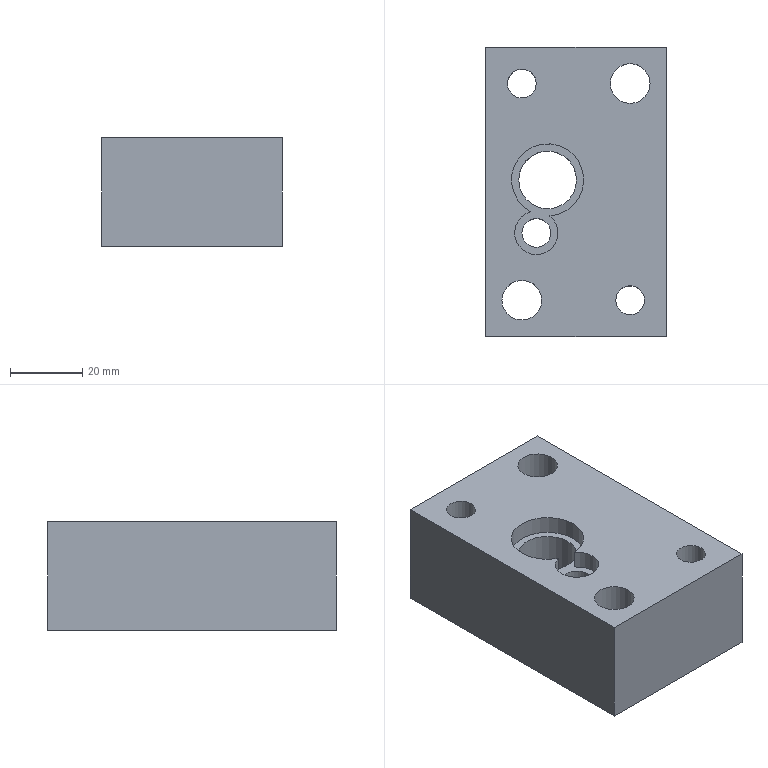Part | NX | features solid 2 | 1 solid | 19 faces | box 50 x 80 x 30 mm | volume 98922 mm3 | cylinder 10 | plane 9 | commonest cylinder face diameters 8 x3 11 x2 17 x2 12 x1 16 x1 20 x1
STEP:
#1=CARTESIAN_POINT('',(535.024,173.652,32.));
#2=VERTEX_POINT('',#1);
#3=CARTESIAN_POINT('',(539.024,173.652,32.));
#4=DIRECTION('',(0.,0.,-1.));
#5=DIRECTION('',(-1.,0.,0.));
#6=AXIS2_PLACEMENT_3D('',#3,#4,#5);
#7=CIRCLE('',#6,4.);
#8=EDGE_CURVE('',#2,#2,#7,.F.);
#9=ORIENTED_EDGE('',*,*,#8,.T.);
#10=EDGE_LOOP('',(#9));
#11=FACE_BOUND('',#10,.T.);
#12=CARTESIAN_POINT('',(556.5,215.,32.));
#13=VERTEX_POINT('',#12);
#14=CARTESIAN_POINT('',(565.,215.,32.));
#15=DIRECTION('',(0.,0.,-1.));
#16=DIRECTION('',(-1.,0.,0.));
#17=AXIS2_PLACEMENT_3D('',#14,#15,#16);
#18=CIRCLE('',#17,8.5);
#19=EDGE_CURVE('',#13,#13,#18,.T.);
#20=ORIENTED_EDGE('',*,*,#19,.F.);
#21=EDGE_LOOP('',(#20));
#22=FACE_BOUND('',#21,.T.);
#23=CARTESIAN_POINT('',(526.5,155.,32.));
#24=VERTEX_POINT('',#23);
#25=CARTESIAN_POINT('',(535.,155.,32.));
#26=DIRECTION('',(0.,0.,-1.));
#27=DIRECTION('',(-1.,0.,0.));
#28=AXIS2_PLACEMENT_3D('',#25,#26,#27);
#29=CIRCLE('',#28,8.5);
#30=EDGE_CURVE('',#24,#24,#29,.T.);
#31=ORIENTED_EDGE('',*,*,#30,.F.);
#32=EDGE_LOOP('',(#31));
#33=FACE_BOUND('',#32,.T.);
#34=CARTESIAN_POINT('',(531.,215.,32.));
#35=VERTEX_POINT('',#34);
#36=CARTESIAN_POINT('',(535.,215.,32.));
#37=DIRECTION('',(0.,0.,-1.));
#38=DIRECTION('',(-1.,0.,0.));
#39=AXIS2_PLACEMENT_3D('',#36,#37,#38);
#40=CIRCLE('',#39,4.);
#41=EDGE_CURVE('',#35,#35,#40,.T.);
#42=ORIENTED_EDGE('',*,*,#41,.F.);
#43=EDGE_LOOP('',(#42));
#44=FACE_BOUND('',#43,.T.);
#45=CARTESIAN_POINT('',(561.,155.,32.));
#46=VERTEX_POINT('',#45);
#47=CARTESIAN_POINT('',(565.,155.,32.));
#48=DIRECTION('',(0.,0.,-1.));
#49=DIRECTION('',(-1.,0.,0.));
#50=AXIS2_PLACEMENT_3D('',#47,#48,#49);
#51=CIRCLE('',#50,4.);
#52=EDGE_CURVE('',#46,#46,#51,.T.);
#53=ORIENTED_EDGE('',*,*,#52,.F.);
#54=EDGE_LOOP('',(#53));
#55=FACE_BOUND('',#54,.T.);
#56=CARTESIAN_POINT('',(575.,225.,32.));
#57=VERTEX_POINT('',#56);
#58=CARTESIAN_POINT('',(525.,225.,32.));
#59=VERTEX_POINT('',#58);
#60=CARTESIAN_POINT('',(590.,225.,32.));
#61=DIRECTION('',(-1.,0.,0.));
#62=VECTOR('',#61,1000.);
#63=LINE('',#60,#62);
#64=EDGE_CURVE('',#57,#59,#63,.T.);
#65=ORIENTED_EDGE('',*,*,#64,.F.);
#66=CARTESIAN_POINT('',(575.,145.,32.));
#67=VERTEX_POINT('',#66);
#68=CARTESIAN_POINT('',(575.,210.,32.));
#69=DIRECTION('',(0.,1.,0.));
#70=VECTOR('',#69,1000.);
#71=LINE('',#68,#70);
#72=EDGE_CURVE('',#67,#57,#71,.T.);
#73=ORIENTED_EDGE('',*,*,#72,.F.);
#74=CARTESIAN_POINT('',(525.,145.,32.));
#75=VERTEX_POINT('',#74);
#76=CARTESIAN_POINT('',(590.,145.,32.));
#77=DIRECTION('',(1.,0.,0.));
#78=VECTOR('',#77,1000.);
#79=LINE('',#76,#78);
#80=EDGE_CURVE('',#75,#67,#79,.T.);
#81=ORIENTED_EDGE('',*,*,#80,.F.);
#82=CARTESIAN_POINT('',(525.,210.,32.));
#83=DIRECTION('',(0.,-1.,0.));
#84=VECTOR('',#83,1000.);
#85=LINE('',#82,#84);
#86=EDGE_CURVE('',#59,#75,#85,.T.);
#87=ORIENTED_EDGE('',*,*,#86,.F.);
#88=EDGE_LOOP('',(#65,#73,#81,#87));
#89=FACE_BOUND('',#88,.T.);
#90=CARTESIAN_POINT('',(534.144,188.315,32.));
#91=VERTEX_POINT('',#90);
#92=CARTESIAN_POINT('',(542.144,188.315,32.));
#93=DIRECTION('',(0.,0.,-1.));
#94=DIRECTION('',(-1.,0.,0.));
#95=AXIS2_PLACEMENT_3D('',#92,#93,#94);
#96=CIRCLE('',#95,8.);
#97=EDGE_CURVE('',#91,#91,#96,.F.);
#98=ORIENTED_EDGE('',*,*,#97,.T.);
#99=EDGE_LOOP('',(#98));
#100=FACE_BOUND('',#99,.T.);
#101=CARTESIAN_POINT('',(590.,210.,32.));
#102=DIRECTION('',(0.,0.,-1.));
#103=DIRECTION('',(1.,0.,0.));
#104=AXIS2_PLACEMENT_3D('',#101,#102,#103);
#105=PLANE('',#104);
#106=ADVANCED_FACE('',(#11,#22,#33,#44,#55,#89,#100),#105,.T.);
#107=CARTESIAN_POINT('',(575.,145.,62.));
#108=VERTEX_POINT('',#107);
#109=CARTESIAN_POINT('',(575.,225.,62.));
#110=VERTEX_POINT('',#109);
#111=CARTESIAN_POINT('',(575.,188.315,62.));
#112=DIRECTION('',(0.,-1.,0.));
#113=VECTOR('',#112,1000.);
#114=LINE('',#111,#113);
#115=EDGE_CURVE('',#108,#110,#114,.F.);
#116=ORIENTED_EDGE('',*,*,#115,.F.);
#117=CARTESIAN_POINT('',(575.,145.,36.));
#118=DIRECTION('',(0.,0.,1.));
#119=VECTOR('',#118,1000.);
#120=LINE('',#117,#119);
#121=EDGE_CURVE('',#67,#108,#120,.T.);
#122=ORIENTED_EDGE('',*,*,#121,.F.);
#123=ORIENTED_EDGE('',*,*,#72,.T.);
#124=CARTESIAN_POINT('',(575.,225.,36.));
#125=DIRECTION('',(0.,0.,1.));
#126=VECTOR('',#125,1000.);
#127=LINE('',#124,#126);
#128=EDGE_CURVE('',#57,#110,#127,.T.);
#129=ORIENTED_EDGE('',*,*,#128,.T.);
#130=EDGE_LOOP('',(#116,#122,#123,#129));
#131=FACE_BOUND('',#130,.T.);
#132=CARTESIAN_POINT('',(575.,160.,36.));
#133=DIRECTION('',(-1.,0.,0.));
#134=DIRECTION('',(0.,0.,-1.));
#135=AXIS2_PLACEMENT_3D('',#132,#133,#134);
#136=PLANE('',#135);
#137=ADVANCED_FACE('',(#131),#136,.F.);
#138=CARTESIAN_POINT('',(525.,225.,62.));
#139=VERTEX_POINT('',#138);
#140=CARTESIAN_POINT('',(542.144,225.,62.));
#141=DIRECTION('',(1.,0.,0.));
#142=VECTOR('',#141,1000.);
#143=LINE('',#140,#142);
#144=EDGE_CURVE('',#110,#139,#143,.F.);
#145=ORIENTED_EDGE('',*,*,#144,.F.);
#146=ORIENTED_EDGE('',*,*,#128,.F.);
#147=ORIENTED_EDGE('',*,*,#64,.T.);
#148=CARTESIAN_POINT('',(525.,225.,36.));
#149=DIRECTION('',(0.,0.,1.));
#150=VECTOR('',#149,1000.);
#151=LINE('',#148,#150);
#152=EDGE_CURVE('',#59,#139,#151,.T.);
#153=ORIENTED_EDGE('',*,*,#152,.T.);
#154=EDGE_LOOP('',(#145,#146,#147,#153));
#155=FACE_BOUND('',#154,.T.);
#156=CARTESIAN_POINT('',(590.,225.,36.));
#157=DIRECTION('',(0.,-1.,0.));
#158=DIRECTION('',(0.,0.,-1.));
#159=AXIS2_PLACEMENT_3D('',#156,#157,#158);
#160=PLANE('',#159);
#161=ADVANCED_FACE('',(#155),#160,.F.);
#162=ORIENTED_EDGE('',*,*,#86,.T.);
#163=CARTESIAN_POINT('',(525.,145.,62.));
#164=VERTEX_POINT('',#163);
#165=CARTESIAN_POINT('',(525.,145.,36.));
#166=DIRECTION('',(0.,0.,1.));
#167=VECTOR('',#166,1000.);
#168=LINE('',#165,#167);
#169=EDGE_CURVE('',#75,#164,#168,.T.);
#170=ORIENTED_EDGE('',*,*,#169,.T.);
#171=CARTESIAN_POINT('',(525.,188.315,62.));
#172=DIRECTION('',(0.,1.,0.));
#173=VECTOR('',#172,1000.);
#174=LINE('',#171,#173);
#175=EDGE_CURVE('',#139,#164,#174,.F.);
#176=ORIENTED_EDGE('',*,*,#175,.F.);
#177=ORIENTED_EDGE('',*,*,#152,.F.);
#178=EDGE_LOOP('',(#162,#170,#176,#177));
#179=FACE_BOUND('',#178,.T.);
#180=CARTESIAN_POINT('',(525.,210.,36.));
#181=DIRECTION('',(1.,0.,0.));
#182=DIRECTION('',(0.,0.,1.));
#183=AXIS2_PLACEMENT_3D('',#180,#181,#182);
#184=PLANE('',#183);
#185=ADVANCED_FACE('',(#179),#184,.F.);
#186=CARTESIAN_POINT('',(542.144,145.,62.));
#187=DIRECTION('',(-1.,0.,0.));
#188=VECTOR('',#187,1000.);
#189=LINE('',#186,#188);
#190=EDGE_CURVE('',#164,#108,#189,.F.);
#191=ORIENTED_EDGE('',*,*,#190,.F.);
#192=ORIENTED_EDGE('',*,*,#169,.F.);
#193=ORIENTED_EDGE('',*,*,#80,.T.);
#194=ORIENTED_EDGE('',*,*,#121,.T.);
#195=EDGE_LOOP('',(#191,#192,#193,#194));
#196=FACE_BOUND('',#195,.T.);
#197=CARTESIAN_POINT('',(535.,145.,36.));
#198=DIRECTION('',(0.,1.,0.));
#199=DIRECTION('',(0.,0.,1.));
#200=AXIS2_PLACEMENT_3D('',#197,#198,#199);
#201=PLANE('',#200);
#202=ADVANCED_FACE('',(#196),#201,.F.);
#203=CARTESIAN_POINT('',(537.504,179.457,62.));
#204=VERTEX_POINT('',#203);
#205=CARTESIAN_POINT('',(542.775,178.335,62.));
#206=VERTEX_POINT('',#205);
#207=CARTESIAN_POINT('',(539.024,173.652,62.));
#208=DIRECTION('',(0.,0.,1.));
#209=DIRECTION('',(1.,0.,0.));
#210=AXIS2_PLACEMENT_3D('',#207,#208,#209);
#211=CIRCLE('',#210,6.);
#212=EDGE_CURVE('',#204,#206,#211,.T.);
#213=ORIENTED_EDGE('',*,*,#212,.F.);
#214=CARTESIAN_POINT('',(542.144,188.315,62.));
#215=DIRECTION('',(0.,0.,1.));
#216=DIRECTION('',(1.,0.,0.));
#217=AXIS2_PLACEMENT_3D('',#214,#215,#216);
#218=CIRCLE('',#217,10.);
#219=EDGE_CURVE('',#206,#204,#218,.T.);
#220=ORIENTED_EDGE('',*,*,#219,.F.);
#221=EDGE_LOOP('',(#213,#220));
#222=FACE_BOUND('',#221,.T.);
#223=CARTESIAN_POINT('',(570.5,215.,62.));
#224=VERTEX_POINT('',#223);
#225=CARTESIAN_POINT('',(565.,215.,62.));
#226=DIRECTION('',(0.,0.,1.));
#227=DIRECTION('',(1.,0.,0.));
#228=AXIS2_PLACEMENT_3D('',#225,#226,#227);
#229=CIRCLE('',#228,5.5);
#230=EDGE_CURVE('',#224,#224,#229,.T.);
#231=ORIENTED_EDGE('',*,*,#230,.F.);
#232=EDGE_LOOP('',(#231));
#233=FACE_BOUND('',#232,.T.);
#234=CARTESIAN_POINT('',(540.5,155.,62.));
#235=VERTEX_POINT('',#234);
#236=CARTESIAN_POINT('',(535.,155.,62.));
#237=DIRECTION('',(0.,0.,1.));
#238=DIRECTION('',(1.,0.,0.));
#239=AXIS2_PLACEMENT_3D('',#236,#237,#238);
#240=CIRCLE('',#239,5.5);
#241=EDGE_CURVE('',#235,#235,#240,.T.);
#242=ORIENTED_EDGE('',*,*,#241,.F.);
#243=EDGE_LOOP('',(#242));
#244=FACE_BOUND('',#243,.T.);
#245=CARTESIAN_POINT('',(539.,215.,62.));
#246=VERTEX_POINT('',#245);
#247=CARTESIAN_POINT('',(535.,215.,62.));
#248=DIRECTION('',(0.,0.,1.));
#249=DIRECTION('',(1.,0.,0.));
#250=AXIS2_PLACEMENT_3D('',#247,#248,#249);
#251=CIRCLE('',#250,4.);
#252=EDGE_CURVE('',#246,#246,#251,.T.);
#253=ORIENTED_EDGE('',*,*,#252,.F.);
#254=EDGE_LOOP('',(#253));
#255=FACE_BOUND('',#254,.T.);
#256=CARTESIAN_POINT('',(569.,155.,62.));
#257=VERTEX_POINT('',#256);
#258=CARTESIAN_POINT('',(565.,155.,62.));
#259=DIRECTION('',(0.,0.,1.));
#260=DIRECTION('',(1.,0.,0.));
#261=AXIS2_PLACEMENT_3D('',#258,#259,#260);
#262=CIRCLE('',#261,4.);
#263=EDGE_CURVE('',#257,#257,#262,.T.);
#264=ORIENTED_EDGE('',*,*,#263,.F.);
#265=EDGE_LOOP('',(#264));
#266=FACE_BOUND('',#265,.T.);
#267=ORIENTED_EDGE('',*,*,#175,.T.);
#268=ORIENTED_EDGE('',*,*,#190,.T.);
#269=ORIENTED_EDGE('',*,*,#115,.T.);
#270=ORIENTED_EDGE('',*,*,#144,.T.);
#271=EDGE_LOOP('',(#267,#268,#269,#270));
#272=FACE_BOUND('',#271,.T.);
#273=CARTESIAN_POINT('',(542.144,188.315,62.));
#274=DIRECTION('',(0.,0.,1.));
#275=DIRECTION('',(1.,0.,0.));
#276=AXIS2_PLACEMENT_3D('',#273,#274,#275);
#277=PLANE('',#276);
#278=ADVANCED_FACE('',(#222,#233,#244,#255,#266,#272),#277,.T.);
#279=ORIENTED_EDGE('',*,*,#263,.T.);
#280=EDGE_LOOP('',(#279));
#281=FACE_BOUND('',#280,.T.);
#282=ORIENTED_EDGE('',*,*,#52,.T.);
#283=EDGE_LOOP('',(#282));
#284=FACE_BOUND('',#283,.T.);
#285=CARTESIAN_POINT('',(565.,155.,86.));
#286=DIRECTION('',(0.,0.,1.));
#287=DIRECTION('',(-1.,0.,0.));
#288=AXIS2_PLACEMENT_3D('',#285,#286,#287);
#289=CYLINDRICAL_SURFACE('',#288,4.);
#290=ADVANCED_FACE('',(#281,#284),#289,.F.);
#291=ORIENTED_EDGE('',*,*,#252,.T.);
#292=EDGE_LOOP('',(#291));
#293=FACE_BOUND('',#292,.T.);
#294=ORIENTED_EDGE('',*,*,#41,.T.);
#295=EDGE_LOOP('',(#294));
#296=FACE_BOUND('',#295,.T.);
#297=CARTESIAN_POINT('',(535.,215.,86.));
#298=DIRECTION('',(0.,0.,1.));
#299=DIRECTION('',(-1.,0.,0.));
#300=AXIS2_PLACEMENT_3D('',#297,#298,#299);
#301=CYLINDRICAL_SURFACE('',#300,4.);
#302=ADVANCED_FACE('',(#293,#296),#301,.F.);
#303=CARTESIAN_POINT('',(540.5,155.,47.));
#304=VERTEX_POINT('',#303);
#305=CARTESIAN_POINT('',(535.,155.,47.));
#306=DIRECTION('',(0.,0.,1.));
#307=DIRECTION('',(1.,0.,0.));
#308=AXIS2_PLACEMENT_3D('',#305,#306,#307);
#309=CIRCLE('',#308,5.5);
#310=EDGE_CURVE('',#304,#304,#309,.F.);
#311=ORIENTED_EDGE('',*,*,#310,.T.);
#312=EDGE_LOOP('',(#311));
#313=FACE_BOUND('',#312,.T.);
#314=ORIENTED_EDGE('',*,*,#241,.T.);
#315=EDGE_LOOP('',(#314));
#316=FACE_BOUND('',#315,.T.);
#317=CARTESIAN_POINT('',(535.,155.,86.));
#318=DIRECTION('',(0.,0.,1.));
#319=DIRECTION('',(-1.,0.,0.));
#320=AXIS2_PLACEMENT_3D('',#317,#318,#319);
#321=CYLINDRICAL_SURFACE('',#320,5.5);
#322=ADVANCED_FACE('',(#313,#316),#321,.F.);
#323=ORIENTED_EDGE('',*,*,#310,.F.);
#324=EDGE_LOOP('',(#323));
#325=FACE_BOUND('',#324,.T.);
#326=CARTESIAN_POINT('',(543.5,155.,47.));
#327=VERTEX_POINT('',#326);
#328=CARTESIAN_POINT('',(535.,155.,47.));
#329=DIRECTION('',(0.,0.,1.));
#330=DIRECTION('',(1.,0.,0.));
#331=AXIS2_PLACEMENT_3D('',#328,#329,#330);
#332=CIRCLE('',#331,8.5);
#333=EDGE_CURVE('',#327,#327,#332,.F.);
#334=ORIENTED_EDGE('',*,*,#333,.T.);
#335=EDGE_LOOP('',(#334));
#336=FACE_BOUND('',#335,.T.);
#337=CARTESIAN_POINT('',(535.,155.,47.));
#338=DIRECTION('',(0.,0.,1.));
#339=DIRECTION('',(-1.,0.,0.));
#340=AXIS2_PLACEMENT_3D('',#337,#338,#339);
#341=PLANE('',#340);
#342=ADVANCED_FACE('',(#325,#336),#341,.F.);
#343=ORIENTED_EDGE('',*,*,#333,.F.);
#344=EDGE_LOOP('',(#343));
#345=FACE_BOUND('',#344,.T.);
#346=ORIENTED_EDGE('',*,*,#30,.T.);
#347=EDGE_LOOP('',(#346));
#348=FACE_BOUND('',#347,.T.);
#349=CARTESIAN_POINT('',(535.,155.,36.));
#350=DIRECTION('',(0.,0.,1.));
#351=DIRECTION('',(-1.,0.,0.));
#352=AXIS2_PLACEMENT_3D('',#349,#350,#351);
#353=CYLINDRICAL_SURFACE('',#352,8.5);
#354=ADVANCED_FACE('',(#345,#348),#353,.F.);
#355=CARTESIAN_POINT('',(570.5,215.,47.));
#356=VERTEX_POINT('',#355);
#357=CARTESIAN_POINT('',(565.,215.,47.));
#358=DIRECTION('',(0.,0.,1.));
#359=DIRECTION('',(1.,0.,0.));
#360=AXIS2_PLACEMENT_3D('',#357,#358,#359);
#361=CIRCLE('',#360,5.5);
#362=EDGE_CURVE('',#356,#356,#361,.F.);
#363=ORIENTED_EDGE('',*,*,#362,.T.);
#364=EDGE_LOOP('',(#363));
#365=FACE_BOUND('',#364,.T.);
#366=ORIENTED_EDGE('',*,*,#230,.T.);
#367=EDGE_LOOP('',(#366));
#368=FACE_BOUND('',#367,.T.);
#369=CARTESIAN_POINT('',(565.,215.,86.));
#370=DIRECTION('',(0.,0.,1.));
#371=DIRECTION('',(-1.,0.,0.));
#372=AXIS2_PLACEMENT_3D('',#369,#370,#371);
#373=CYLINDRICAL_SURFACE('',#372,5.5);
#374=ADVANCED_FACE('',(#365,#368),#373,.F.);
#375=ORIENTED_EDGE('',*,*,#362,.F.);
#376=EDGE_LOOP('',(#375));
#377=FACE_BOUND('',#376,.T.);
#378=CARTESIAN_POINT('',(573.5,215.,47.));
#379=VERTEX_POINT('',#378);
#380=CARTESIAN_POINT('',(565.,215.,47.));
#381=DIRECTION('',(0.,0.,1.));
#382=DIRECTION('',(1.,0.,0.));
#383=AXIS2_PLACEMENT_3D('',#380,#381,#382);
#384=CIRCLE('',#383,8.5);
#385=EDGE_CURVE('',#379,#379,#384,.F.);
#386=ORIENTED_EDGE('',*,*,#385,.T.);
#387=EDGE_LOOP('',(#386));
#388=FACE_BOUND('',#387,.T.);
#389=CARTESIAN_POINT('',(565.,215.,47.));
#390=DIRECTION('',(0.,0.,1.));
#391=DIRECTION('',(-1.,0.,0.));
#392=AXIS2_PLACEMENT_3D('',#389,#390,#391);
#393=PLANE('',#392);
#394=ADVANCED_FACE('',(#377,#388),#393,.F.);
#395=ORIENTED_EDGE('',*,*,#385,.F.);
#396=EDGE_LOOP('',(#395));
#397=FACE_BOUND('',#396,.T.);
#398=ORIENTED_EDGE('',*,*,#19,.T.);
#399=EDGE_LOOP('',(#398));
#400=FACE_BOUND('',#399,.T.);
#401=CARTESIAN_POINT('',(565.,215.,36.));
#402=DIRECTION('',(0.,0.,1.));
#403=DIRECTION('',(-1.,0.,0.));
#404=AXIS2_PLACEMENT_3D('',#401,#402,#403);
#405=CYLINDRICAL_SURFACE('',#404,8.5);
#406=ADVANCED_FACE('',(#397,#400),#405,.F.);
#407=ORIENTED_EDGE('',*,*,#8,.F.);
#408=EDGE_LOOP('',(#407));
#409=FACE_BOUND('',#408,.T.);
#410=CARTESIAN_POINT('',(543.024,173.652,57.));
#411=VERTEX_POINT('',#410);
#412=CARTESIAN_POINT('',(539.024,173.652,57.));
#413=DIRECTION('',(0.,0.,1.));
#414=DIRECTION('',(1.,0.,0.));
#415=AXIS2_PLACEMENT_3D('',#412,#413,#414);
#416=CIRCLE('',#415,4.);
#417=EDGE_CURVE('',#411,#411,#416,.T.);
#418=ORIENTED_EDGE('',*,*,#417,.T.);
#419=EDGE_LOOP('',(#418));
#420=FACE_BOUND('',#419,.T.);
#421=CARTESIAN_POINT('',(539.024,173.652,62.));
#422=DIRECTION('',(0.,0.,-1.));
#423=DIRECTION('',(-1.,0.,0.));
#424=AXIS2_PLACEMENT_3D('',#421,#422,#423);
#425=CYLINDRICAL_SURFACE('',#424,4.);
#426=ADVANCED_FACE('',(#409,#420),#425,.F.);
#427=CARTESIAN_POINT('',(537.504,179.457,57.));
#428=VERTEX_POINT('',#427);
#429=CARTESIAN_POINT('',(542.775,178.335,57.));
#430=VERTEX_POINT('',#429);
#431=CARTESIAN_POINT('',(539.024,173.652,57.));
#432=DIRECTION('',(0.,0.,1.));
#433=DIRECTION('',(1.,0.,0.));
#434=AXIS2_PLACEMENT_3D('',#431,#432,#433);
#435=CIRCLE('',#434,6.);
#436=EDGE_CURVE('',#428,#430,#435,.T.);
#437=ORIENTED_EDGE('',*,*,#436,.T.);
#438=CARTESIAN_POINT('',(542.144,188.315,57.));
#439=DIRECTION('',(0.,0.,1.));
#440=DIRECTION('',(1.,0.,0.));
#441=AXIS2_PLACEMENT_3D('',#438,#439,#440);
#442=CIRCLE('',#441,10.);
#443=EDGE_CURVE('',#430,#428,#442,.T.);
#444=ORIENTED_EDGE('',*,*,#443,.T.);
#445=EDGE_LOOP('',(#437,#444));
#446=FACE_BOUND('',#445,.T.);
#447=ORIENTED_EDGE('',*,*,#417,.F.);
#448=EDGE_LOOP('',(#447));
#449=FACE_BOUND('',#448,.T.);
#450=CARTESIAN_POINT('',(550.144,188.315,57.));
#451=VERTEX_POINT('',#450);
#452=CARTESIAN_POINT('',(542.144,188.315,57.));
#453=DIRECTION('',(0.,0.,1.));
#454=DIRECTION('',(1.,0.,0.));
#455=AXIS2_PLACEMENT_3D('',#452,#453,#454);
#456=CIRCLE('',#455,8.);
#457=EDGE_CURVE('',#451,#451,#456,.T.);
#458=ORIENTED_EDGE('',*,*,#457,.F.);
#459=EDGE_LOOP('',(#458));
#460=FACE_BOUND('',#459,.T.);
#461=CARTESIAN_POINT('',(539.024,173.652,57.));
#462=DIRECTION('',(0.,0.,1.));
#463=DIRECTION('',(1.,0.,0.));
#464=AXIS2_PLACEMENT_3D('',#461,#462,#463);
#465=PLANE('',#464);
#466=ADVANCED_FACE('',(#446,#449,#460),#465,.T.);
#467=ORIENTED_EDGE('',*,*,#436,.F.);
#468=CARTESIAN_POINT('',(537.504,179.457,57.));
#469=DIRECTION('',(0.,0.,1.));
#470=VECTOR('',#469,1000.);
#471=LINE('',#468,#470);
#472=EDGE_CURVE('',#428,#204,#471,.T.);
#473=ORIENTED_EDGE('',*,*,#472,.T.);
#474=ORIENTED_EDGE('',*,*,#212,.T.);
#475=CARTESIAN_POINT('',(542.775,178.335,62.));
#476=DIRECTION('',(0.,0.,1.));
#477=VECTOR('',#476,1000.);
#478=LINE('',#475,#477);
#479=EDGE_CURVE('',#206,#430,#478,.F.);
#480=ORIENTED_EDGE('',*,*,#479,.T.);
#481=EDGE_LOOP('',(#467,#473,#474,#480));
#482=FACE_BOUND('',#481,.T.);
#483=CARTESIAN_POINT('',(539.024,173.652,57.));
#484=DIRECTION('',(0.,0.,1.));
#485=DIRECTION('',(1.,0.,0.));
#486=AXIS2_PLACEMENT_3D('',#483,#484,#485);
#487=CYLINDRICAL_SURFACE('',#486,6.);
#488=ADVANCED_FACE('',(#482),#487,.F.);
#489=ORIENTED_EDGE('',*,*,#443,.F.);
#490=ORIENTED_EDGE('',*,*,#479,.F.);
#491=ORIENTED_EDGE('',*,*,#219,.T.);
#492=ORIENTED_EDGE('',*,*,#472,.F.);
#493=EDGE_LOOP('',(#489,#490,#491,#492));
#494=FACE_BOUND('',#493,.T.);
#495=CARTESIAN_POINT('',(542.144,188.315,57.));
#496=DIRECTION('',(0.,0.,1.));
#497=DIRECTION('',(1.,0.,0.));
#498=AXIS2_PLACEMENT_3D('',#495,#496,#497);
#499=CYLINDRICAL_SURFACE('',#498,10.);
#500=ADVANCED_FACE('',(#494),#499,.F.);
#501=ORIENTED_EDGE('',*,*,#97,.F.);
#502=EDGE_LOOP('',(#501));
#503=FACE_BOUND('',#502,.T.);
#504=ORIENTED_EDGE('',*,*,#457,.T.);
#505=EDGE_LOOP('',(#504));
#506=FACE_BOUND('',#505,.T.);
#507=CARTESIAN_POINT('',(542.144,188.315,62.));
#508=DIRECTION('',(0.,0.,-1.));
#509=DIRECTION('',(-1.,0.,0.));
#510=AXIS2_PLACEMENT_3D('',#507,#508,#509);
#511=CYLINDRICAL_SURFACE('',#510,8.);
#512=ADVANCED_FACE('',(#503,#506),#511,.F.);
#513=CLOSED_SHELL('',(#106,#137,#161,#185,#202,#278,#290,#302,#322,#342,#354,#374,#394,#406,#426,#466,#488,#500,#512));
#514=MANIFOLD_SOLID_BREP('',#513);
#515=(LENGTH_UNIT()NAMED_UNIT(*)SI_UNIT(.MILLI.,.METRE.));
#516=UNCERTAINTY_MEASURE_WITH_UNIT(LENGTH_MEASURE(0.00001),#515,'','');
#517=(NAMED_UNIT(*)PLANE_ANGLE_UNIT()SI_UNIT($,.RADIAN.));
#518=(NAMED_UNIT(*)SI_UNIT($,.STERADIAN.)SOLID_ANGLE_UNIT());
#519=(GEOMETRIC_REPRESENTATION_CONTEXT(3)GLOBAL_UNCERTAINTY_ASSIGNED_CONTEXT((#516))GLOBAL_UNIT_ASSIGNED_CONTEXT((#515,#517,#518))REPRESENTATION_CONTEXT('',''));
#520=ADVANCED_BREP_SHAPE_REPRESENTATION('',(#514),#519);